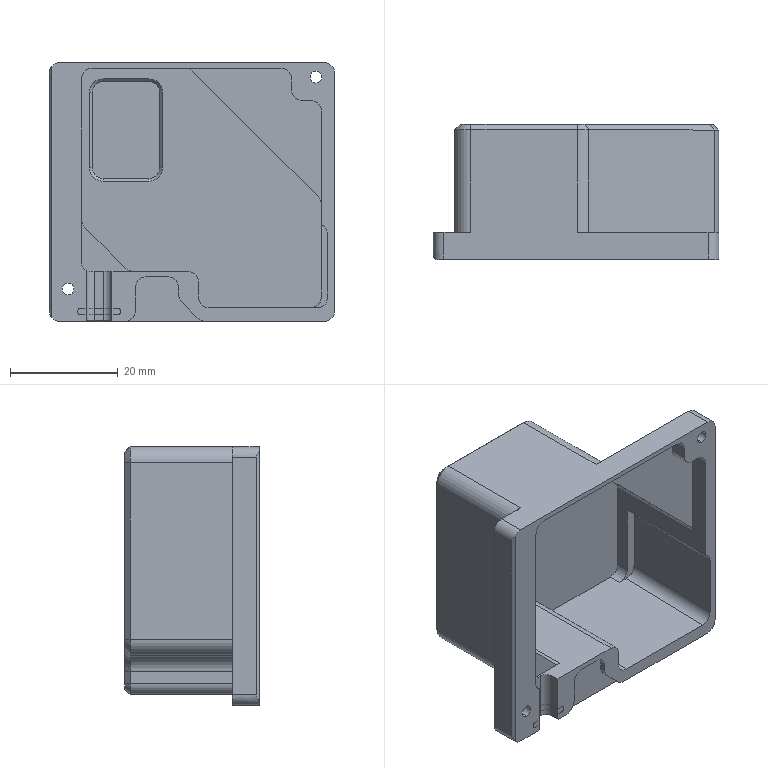NC program | NX | posted with a generic post | part box 53 x 25 x 48 mm
Whole program:
N10 G17 G21 G94 G90
(ZLEVEL_PROFILE_STEEP , TOOL : D4-12-D4-50-3T-ROUGH)
N12 T09 M6
N14 G54
N16 G17 G0 G90 X17.5 Y-7.5 B0. C0. S4000 M3
N18 G43 Z31.374 H9
N20 Z1.115 B-180. C178.5
N22 G94 G1 Z0.115 F1500.
N24 X18.3
N26 G3 X19.5 Y-6.3 R1.2
N28 G1 Y-4.39
N30 Y-3.37 Z0.068
N32 Y-3.297 Z0.065
N34 Y-6.3
N36 Z0.015
N38 Y-3.3
N40 X19.495
N42 X7.834
N44 Z-0.035
N46 X19.495
N48 X19.5
N50 Y-6.3
N52 Z-0.085
N54 Y-3.3
N56 X19.495
N58 X7.835
N60 Z-0.135
N62 X19.495
N64 X19.5
N66 Y-6.3
N68 Z-0.185
N70 Y-3.3
N72 X19.495
N74 X7.836
N76 Z-0.235
N78 X19.495
N80 X19.5
N82 Y-6.3
N84 Z-0.285
N86 Y-3.3
N88 X19.495
N90 X7.837
N92 Z-0.335
N94 X19.495
N96 X19.5
N98 Y-6.3
N100 Z-0.385
N102 Y-3.3
N104 X19.495
N106 X7.838
N108 Z-0.435
N110 X19.495
N112 X19.5
N114 Y-6.3
N116 Z-0.485
N118 Y-3.3
N120 X19.495
N122 X7.839
N124 X7.84 Z-0.535
N126 X19.495
N128 X19.5
N130 Y-6.3
N132 Z-0.585
N134 Y-3.3
N136 X19.495
N138 X7.84
N140 X7.841 Z-0.634
N142 X19.495
N144 X19.5
N146 Y-6.3
N148 Z-0.684
N150 Y-3.3
N152 X19.495
N154 X7.841
N156 X7.842 Z-0.734
N158 X19.495
N160 X19.5
N162 Y-6.3
N164 Z-0.784
N166 Y-3.3
N168 X19.495
N170 X7.842
N172 X7.843 Z-0.834
N174 X19.495
N176 X19.5
N178 Y-6.3
N180 Z-0.884
N182 Y-3.3
N184 X19.495
N186 X7.843
N188 X7.844 Z-0.934
N190 X19.495
N192 X19.5
N194 Y-6.3
N196 Z-0.984
N198 Y-3.3
N200 X19.495
N202 X7.844
N204 X7.845 Z-1.034
N206 X19.495
N208 X19.5
N210 Y-6.3
N212 Z-1.084
N214 Y-3.3
N216 X19.495
N218 X7.845
N220 X7.846 Z-1.134
N222 X19.495
N224 X19.5
N226 Y-6.3
N228 Z-1.184
N230 Y-3.3
N232 X19.495
N234 X7.847
N236 Z-1.234
N238 X19.495
N240 X19.5
N242 Y-6.3
N244 Z-1.284
N246 Y-3.3
N248 X19.495
N250 X7.848
N252 Z-1.334
N254 X19.495
N256 X19.5
N258 Y-6.3
N260 Z-1.384
N262 Y-3.3
N264 X19.495
N266 X7.849
N268 Z-1.434
N270 X19.495
N272 X19.5
N274 Y-6.3
N276 Z-1.484
N278 Y-3.3
N280 X19.495
N282 X7.85
N284 Z-1.534
N286 X19.495
N288 X19.5
N290 Y-6.3
N292 Z-1.584
N294 Y-3.3
N296 X19.495
N298 X7.851
N300 Z-1.634
N302 X19.495
N304 X19.5
N306 Y-6.3
N308 Z-1.684
N310 Y-3.3
N312 X19.495
N314 X7.852
N316 X7.853 Z-1.734
N318 X19.495
N320 X19.5
N322 Y-6.3
N324 Z-1.784
N326 Y-3.3
N328 X19.495
N330 X7.853
N332 X7.854 Z-1.834
N334 X19.495
N336 X19.5
N338 Y-6.3
N340 Z-1.884
N342 Y-3.3
N344 X19.495
N346 X7.854
N348 X7.855 Z-1.934
N350 X19.495
N352 X19.5
N354 Y-6.3
N356 Z-1.983
N358 Y-3.3
N360 X19.495
N362 X7.855
N364 X7.856 Z-2.033
N366 X19.495
N368 X19.5
N370 Y-6.3
N372 Z-2.083
N374 Y-3.3
N376 X19.495
N378 X7.856
N380 X7.857 Z-2.133
N382 X19.495
N384 X19.5
N386 Y-6.3
N388 Z-2.183
N390 Y-3.3
N392 X19.495
N394 X7.857
N396 X7.858 Z-2.233
N398 X19.495
N400 X19.5 Y-3.301
N402 Y-6.3
N404 Z-2.283
N406 Y-3.301
N408 X19.495 Y-3.3
N410 X7.859
N412 Z-2.333
N414 X19.495
N416 X19.5 Y-3.301
N418 Y-6.3
N420 Z-2.383
N422 Y-3.301
N424 X19.495 Y-3.3
N426 X7.86
N428 Z-2.433
N430 X19.495
N432 X19.5 Y-3.301
N434 Y-6.3
N436 Z-2.483
N438 Y-3.301
N440 X19.495 Y-3.3
N442 X7.861
N444 Z-2.533
N446 X19.495
N448 X19.5 Y-3.301
N450 Y-6.3
N452 Z-2.583
N454 Y-3.301
N456 X19.495 Y-3.3
N458 X7.862
N460 Z-2.633
N462 X19.495
N464 X19.5 Y-3.301
N466 Y-6.3
N468 Z-2.683
N470 Y-3.301
N472 X19.495 Y-3.3
N474 X7.863
N476 Z-2.733
N478 X19.495
N480 X19.5 Y-3.301
N482 Y-6.3
N484 Z-2.783
N486 Y-3.301
N488 X19.495 Y-3.3
N490 X7.864
N492 Z-2.833
N494 X19.495
N496 X19.5 Y-3.301
N498 Y-6.3
N500 Z-2.883
N502 Y-3.301
N504 X19.495 Y-3.3
N506 X7.865
N508 Z-2.933
N510 X19.495
N512 X19.5 Y-3.301
N514 Y-6.3
N516 Z-2.983
N518 Y-3.301
N520 X19.495 Y-3.3
N522 X7.866
N524 Z-3.033
N526 X19.495
N528 X19.5 Y-3.301
N530 Y-6.3
N532 Z-3.083
N534 Y-3.301
N536 X19.495 Y-3.3
N538 X7.867
N540 Z-3.133
N542 X19.495
N544 X19.5 Y-3.301
N546 Y-6.3
N548 Z-3.183
N550 Y-3.301
N552 X19.495 Y-3.3
N554 X7.868
N556 Z-3.233
N558 X19.495
N560 X19.5 Y-3.301
N562 Y-6.3
N564 Z-3.282
N566 Y-3.301
N568 X19.495 Y-3.3
N570 X7.869
N572 Z-3.332
N574 X19.495
N576 X19.5 Y-3.301
N578 Y-6.3
N580 Z-3.382
N582 Y-3.301
N584 X19.495 Y-3.3
N586 X7.87
N588 Z-3.432
N590 X19.495
N592 X19.5 Y-3.301
N594 Y-6.3
N596 Z-3.482
N598 Y-3.301
N600 X19.495 Y-3.3
N602 X7.87
N604 X7.871 Z-3.532
N606 X19.495
N608 X19.5 Y-3.301
N610 Y-6.3
N612 Z-3.582
N614 Y-3.301
N616 X19.495 Y-3.3
N618 X7.871
N620 X7.872 Z-3.632
N622 X19.495
N624 X19.5 Y-3.301
N626 Y-6.3
N628 Z-3.682
N630 Y-3.301
N632 X19.495 Y-3.3
N634 X7.872
N636 X7.873 Z-3.732
N638 X19.495
N640 X19.5 Y-3.301
N642 Y-6.3
N644 Z-3.782
N646 Y-3.301
N648 X19.495 Y-3.3
N650 X7.873
N652 X7.874 Z-3.832
N654 X19.495
N656 X19.5 Y-3.301
N658 Y-6.3
N660 Z-3.882
N662 Y-3.301
N664 X19.495 Y-3.3
N666 X7.874
N668 X7.875 Z-3.932
N670 X19.495
N672 X19.5 Y-3.301
N674 Y-6.3
N676 Z-3.982
N678 Y-3.301
N680 X19.495 Y-3.3
N682 X7.875
N684 X7.876 Z-4.032
N686 X19.495
N688 X19.5 Y-3.301
N690 Y-6.3
N692 Z-4.082
N694 Y-3.301
N696 X19.495 Y-3.3
N698 X7.876
N700 X7.877 Z-4.132
N702 X19.495
N704 X19.5 Y-3.301
N706 Y-6.3
N708 Z-4.182
N710 Y-3.301
N712 X19.495 Y-3.3
N714 X7.877
N716 X7.878 Z-4.232
N718 X19.495
N720 X19.5 Y-3.301
N722 Y-6.3
N724 Z-4.282
N726 Y-3.301
N728 X19.495 Y-3.3
N730 X7.878
N732 X7.879 Z-4.332
N734 X19.495
N736 X19.5 Y-3.301
N738 Y-6.3
N740 Z-4.382
N742 Y-3.301
N744 X19.495 Y-3.3
N746 X7.879
N748 X7.88 Z-4.432
N750 X19.495
N752 X19.5 Y-3.301
N754 Y-6.3
N756 Z-4.482
N758 Y-3.301
N760 X19.495 Y-3.3
N762 X7.88
N764 X7.881 Z-4.532
N766 X19.495
N768 X19.5 Y-3.301
N770 Y-6.3
N772 Z-4.582
N774 Y-3.301
N776 X19.495 Y-3.3
N778 X7.881
N780 X7.882 Z-4.631
N782 X19.495
N784 X19.5 Y-3.301
N786 Y-6.3
N788 Z-4.681
N790 Y-3.301
N792 X19.495 Y-3.3
N794 X7.882
N796 X7.883 Z-4.731
N798 X19.495
N800 X19.5 Y-3.301
N802 Y-6.3
N804 Z-4.781
N806 Y-3.301
N808 X19.495 Y-3.3
N810 X7.883
N812 X7.884 Z-4.831
N814 X19.495
N816 X19.5 Y-3.301
N818 Y-6.3
N820 Z-4.881
N822 Y-3.301
N824 X19.495 Y-3.3
N826 X7.884
N828 X7.885 Z-4.931
N830 X19.495
N832 X19.5 Y-3.301
N834 Y-6.3
N836 Z-4.981
N838 Y-3.301
N840 X19.495 Y-3.3
N842 X7.885
N844 X7.886 Z-5.031
N846 X19.495
N848 X19.5 Y-3.301
N850 Y-6.3
N852 Z-5.081
N854 Y-3.301
N856 X19.495 Y-3.3
N858 X7.886
N860 Z-5.131
N862 X19.495
N864 X19.5 Y-3.301
N866 Y-6.3
N868 Z-5.181
N870 Y-3.301
N872 X19.495 Y-3.3
N874 X7.887
N876 Z-5.231
N878 X19.495
N880 X19.5 Y-3.301
N882 Y-6.3
N884 Z-5.281
N886 Y-3.301
N888 X19.495 Y-3.3
N890 X7.888
N892 Z-5.331
N894 X19.495
N896 X19.5 Y-3.301
N898 Y-6.3
N900 Z-5.381
N902 Y-3.301
N904 X19.495 Y-3.3
N906 X7.889
N908 Z-5.431
N910 X19.495
N912 X19.5 Y-3.301
N914 Y-6.3
N916 Z-5.481
N918 Y-3.301
N920 X19.495 Y-3.3
N922 X7.89
N924 Z-5.531
N926 X19.495
N928 X19.5 Y-3.301
N930 Y-6.3
N932 Z-5.581
N934 Y-3.301
N936 X19.495 Y-3.3
N938 X7.89
N940 X7.891 Z-5.631
N942 X19.495
N944 X19.5 Y-3.301
N946 Y-6.3
N948 Z-5.681
N950 Y-3.301
N952 X19.495 Y-3.3
N954 X7.891
N956 X7.892 Z-5.731
N958 X19.495
N960 X19.5 Y-3.301
N962 Y-6.3
N964 Z-5.781
N966 Y-3.301
N968 X19.495 Y-3.3
N970 X7.892
N972 X7.893 Z-5.831
N974 X19.495
N976 X19.5 Y-3.301
N978 Y-6.3
N980 Z-5.881
N982 Y-3.301
N984 X19.495 Y-3.3
N986 X7.893
N988 X7.894 Z-5.931
N990 X19.495
N992 X19.5 Y-3.301
N994 Y-6.3
N996 Z-5.98
N998 Y-3.301
N1000 X19.495 Y-3.3
N1002 X7.894
N1004 Z-6.03
N1006 X19.495
N1008 X19.5 Y-3.301
N1010 Y-6.3
N1012 Z-6.08
N1014 Y-3.301
N1016 X19.495 Y-3.3
N1018 X7.895
N1020 Z-6.13
N1022 X19.495
N1024 X19.5 Y-3.301
N1026 Y-6.3
N1028 Z-6.18
N1030 Y-3.301
N1032 X19.495 Y-3.3
N1034 X7.896
N1036 Z-6.23
N1038 X19.495
N1040 X19.5 Y-3.301
N1042 Y-6.3
N1044 Z-6.28
N1046 Y-3.301
N1048 X19.495 Y-3.3
N1050 X7.897
N1052 Z-6.33
N1054 X19.495
N1056 X19.5 Y-3.301
N1058 Y-6.3
N1060 Z-6.38
N1062 Y-3.301
N1064 X19.495 Y-3.3
N1066 X7.898
N1068 Z-6.43
N1070 X19.495
N1072 X19.5 Y-3.301
N1074 Y-6.3
N1076 Z-6.48
N1078 Y-3.301
N1080 X19.495 Y-3.3
N1082 X7.898
N1084 X7.899 Z-6.53
N1086 X19.495
N1088 X19.5 Y-3.301
N1090 Y-6.3
N1092 Z-6.58
N1094 Y-3.301
N1096 X19.495 Y-3.3
N1098 X7.899
N1100 X7.9 Z-6.63
N1102 X19.495
N1104 X19.5 Y-3.301
N1106 Y-6.3
N1108 Z-6.68
N1110 Y-3.301
N1112 X19.495 Y-3.3
N1114 X7.9
N1116 X7.901 Z-6.73
N1118 X19.495
N1120 X19.5 Y-3.301
N1122 Y-6.3
N1124 Z-6.78
N1126 Y-3.301
N1128 X19.495 Y-3.3
N1130 X7.901
N1132 X7.902 Z-6.83
N1134 X19.495
N1136 X19.5 Y-3.301
N1138 Y-6.3
N1140 Z-6.88
N1142 Y-3.301
N1144 X19.495 Y-3.3
N1146 X7.902
N1148 Z-6.93
N1150 X19.495
N1152 X19.5 Y-3.301
N1154 Y-6.3
N1156 Z-6.98
N1158 Y-3.301
N1160 X19.495 Y-3.3
N1162 X7.903
N1164 Z-7.03
N1166 X19.495
N1168 X19.5 Y-3.301
N1170 Y-6.3
N1172 Z-7.08
N1174 Y-3.301
N1176 X19.495 Y-3.3
N1178 X7.904
N1180 Z-7.13
N1182 X19.495
N1184 X19.5 Y-3.301
N1186 Y-6.3
N1188 Z-7.18
N1190 Y-3.301
N1192 X19.495 Y-3.3
N1194 X7.905
N1196 Z-7.23
N1198 X19.495
N1200 X19.5 Y-3.301
N1202 Y-6.3
N1204 Z-7.28
N1206 Y-3.301
N1208 X19.495 Y-3.3
N1210 X7.905
N1212 X7.906 Z-7.329
N1214 X19.495
N1216 X19.5 Y-3.301
N1218 Y-6.3
N1220 Z-7.379
N1222 Y-3.301
N1224 X19.495 Y-3.3
N1226 X7.906
N1228 X7.907 Z-7.429
N1230 X19.495
N1232 X19.5 Y-3.301
N1234 Y-6.3
N1236 Z-7.479
N1238 Y-3.301
N1240 X19.495 Y-3.3
N1242 X7.907
N1244 Z-7.529
N1246 X19.495
N1248 X19.5 Y-3.301
N1250 Y-6.3
N1252 Z-7.579
N1254 Y-3.301
N1256 X19.495 Y-3.3
N1258 X7.908
N1260 Z-7.629
N1262 X19.495
N1264 X19.5 Y-3.301
N1266 Y-6.3
N1268 Z-7.679
N1270 Y-3.301
N1272 X19.495 Y-3.3
N1274 X7.909
N1276 Z-7.729
N1278 X19.495
N1280 X19.5 Y-3.301
N1282 Y-6.3
N1284 Z-7.779
N1286 Y-3.301
N1288 X19.495 Y-3.3
N1290 X7.909
N1292 X7.91 Z-7.829
N1294 X19.495
N1296 X19.5 Y-3.301
N1298 Y-6.3
N1300 Z-7.879
N1302 Y-3.301
N1304 X19.495 Y-3.3
N1306 X7.91
N1308 X7.911 Z-7.929
N1310 X19.495
N1312 X19.5 Y-3.301
N1314 Y-6.3
N1316 Z-7.979
N1318 Y-3.301
N1320 X19.495 Y-3.3
N1322 X7.911
N1324 Z-8.029
N1326 X19.495
N1328 X19.5 Y-3.301
N1330 Y-6.3
N1332 Z-8.079
N1334 Y-3.301
N1336 X19.495 Y-3.3
N1338 X7.912
N1340 Z-8.129
N1342 X19.495
N1344 X19.5 Y-3.301
N1346 Y-6.3
N1348 Z-8.179
N1350 Y-3.301
N1352 X19.495 Y-3.3
N1354 X7.913
N1356 Z-8.229
N1358 X19.495
N1360 X19.5 Y-3.301
N1362 Y-6.3
N1364 Z-8.279
N1366 Y-3.301
N1368 X19.495 Y-3.3
N1370 X7.913
N1372 X7.914 Z-8.329
N1374 X19.495
N1376 X19.5 Y-3.301
N1378 Y-6.3
N1380 Z-8.379
N1382 Y-3.301
N1384 X19.495 Y-3.3
N1386 X7.914
N1388 X7.915 Z-8.429
N1390 X19.495
N1392 X19.5 Y-3.301
N1394 Y-6.3
N1396 Z-8.479
N1398 Y-3.301
N1400 X19.495 Y-3.3
N1402 X7.915
N1404 Z-8.529
N1406 X19.495
N1408 X19.5 Y-3.301
N1410 Y-6.3
N1412 Z-8.579
N1414 Y-3.301
N1416 X19.495 Y-3.3
N1418 X7.916
N1420 Z-8.629
N1422 X19.495
N1424 X19.5 Y-3.301
N1426 Y-6.3
N1428 Z-8.678
N1430 Y-3.301
N1432 X19.495 Y-3.3
N1434 X7.917
N1436 Z-8.728
N1438 X19.495
N1440 X19.5 Y-3.301
N1442 Y-6.3
N1444 Z-8.778
N1446 Y-3.301
N1448 X19.495 Y-3.3
N1450 X7.917
N1452 X7.918 Z-8.828
N1454 X19.495
N1456 X19.5 Y-3.301
N1458 Y-6.3
N1460 Z-8.878
N1462 Y-3.301
N1464 X19.495 Y-3.3
N1466 X7.918
N1468 Z-8.928
N1470 X19.495
N1472 X19.5 Y-3.301
N1474 Y-6.3
N1476 Z-8.978
N1478 Y-3.301
N1480 X19.495 Y-3.3
N1482 X7.919
N1484 Z-9.028
N1486 X19.495
N1488 X19.5 Y-3.301
N1490 Y-6.3
N1492 Z-9.078
N1494 Y-3.301
N1496 X19.495 Y-3.3
N1498 X7.92
N1500 Z-9.128
N1502 X19.495
N1504 X19.5 Y-3.301
N1506 Y-6.3
N1508 Z-9.178
N1510 Y-3.301
N1512 X19.495 Y-3.3
N1514 X7.92
N1516 X7.921 Z-9.228
N1518 X19.495
N1520 X19.5 Y-3.301
N1522 Y-6.3
N1524 Z-9.278
N1526 Y-3.301
N1528 X19.495 Y-3.3
N1530 X7.921
N1532 X7.922 Z-9.328
N1534 X19.495
N1536 X19.5 Y-3.301
N1538 Y-6.3
N1540 Z-9.378
N1542 Y-3.301
N1544 X19.495 Y-3.3
N1546 X7.922
N1548 Z-9.428
N1550 X19.495
N1552 X19.5 Y-3.301
N1554 Y-6.3
N1556 Z-9.478
N1558 Y-3.301
N1560 X19.495 Y-3.3
N1562 X7.923
N1564 Z-9.528
N1566 X19.495
N1568 X19.5 Y-3.301
N1570 Y-6.3
N1572 Z-9.578
N1574 Y-3.301
N1576 X19.495 Y-3.3
N1578 X7.924
N1580 Z-9.628
N1582 X19.495
N1584 X19.5 Y-3.301
N1586 Y-6.3
N1588 Z-9.678
N1590 Y-3.301
N1592 X19.495 Y-3.3
N1594 X7.924
N1596 X7.925 Z-9.728
N1598 X19.495
N1600 X19.5 Y-3.301
N1602 Y-6.3
N1604 Z-9.778
N1606 Y-3.301
N1608 X19.495 Y-3.3
N1610 X7.925
N1612 Z-9.828
N1614 X19.495
N1616 X19.5 Y-3.301
N1618 Y-6.3
N1620 Z-9.878
N1622 Y-3.301
N1624 X19.495 Y-3.3
N1626 X7.926
N1628 Z-9.928
N1630 X19.495
N1632 X19.5 Y-3.301
N1634 Y-6.3
N1636 Z-9.977
N1638 Y-3.301
N1640 X19.495 Y-3.3
N1642 X7.927
N1644 Z-10.027
N1646 X19.495
N1648 X19.5 Y-3.301
N1650 Y-6.3
N1652 Z-10.077
N1654 Y-3.301
N1656 X19.495 Y-3.3
N1658 X7.927
N1660 X7.928 Z-10.127
N1662 X19.495
N1664 X19.5 Y-3.301
N1666 Y-6.3
N1668 Z-10.177
N1670 Y-3.301
N1672 X19.495 Y-3.3
N1674 X7.928
N1676 Z-10.227
N1678 X19.495
N1680 X19.5 Y-3.301
N1682 Y-6.3
N1684 Z-10.277
N1686 Y-3.301
N1688 X19.495 Y-3.3
N1690 X7.929
N1692 Z-10.327
N1694 X19.495
N1696 X19.5 Y-3.301
N1698 Y-6.3
N1700 Z-10.377
N1702 Y-3.301
N1704 X19.495 Y-3.3
N1706 X7.929
N1708 X7.93 Z-10.427
N1710 X19.495
N1712 X19.5 Y-3.301
N1714 Y-6.3
N1716 Z-10.477
N1718 Y-3.301
N1720 X19.495 Y-3.3
N1722 X7.93
N1724 Z-10.527
N1726 X19.495
N1728 X19.5 Y-3.301
N1730 Y-6.3
N1732 Z-10.577
N1734 Y-3.301
N1736 X19.495 Y-3.3
N1738 X7.931
N1740 Z-10.627
N1742 X19.495
N1744 X19.5 Y-3.301
N1746 Y-6.3
N1748 Z-10.677
N1750 Y-3.301
N1752 X19.495 Y-3.3
N1754 X7.931
N1756 X7.932 Z-10.727
N1758 X19.495
N1760 X19.5 Y-3.301
N1762 Y-6.3
N1764 Z-10.777
N1766 Y-3.301
N1768 X19.495 Y-3.3
N1770 X7.932
N1772 X7.933 Z-10.827
N1774 X19.495
N1776 X19.5 Y-3.301
N1778 Y-6.3
N1780 Z-10.877
N1782 Y-3.301
N1784 X19.495 Y-3.3
N1786 X7.933
N1788 Z-10.927
N1790 X19.495
N1792 X19.5 Y-3.301
N1794 Y-6.3
N1796 Z-10.977
N1798 Y-3.301
N1800 X19.495 Y-3.3
N1802 X7.934
N1804 Z-11.027
N1806 X19.495
N1808 X19.5 Y-3.301
N1810 Y-6.3
N1812 Z-11.077
N1814 Y-3.301
N1816 X19.495 Y-3.3
N1818 X7.934
N1820 X7.935 Z-11.127
N1822 X19.495
N1824 X19.5 Y-3.301
N1826 Y-6.3
N1828 Z-11.177
N1830 Y-3.301
N1832 X19.495 Y-3.3
N1834 X7.935
N1836 Z-11.227
N1838 X19.495
N1840 X19.5 Y-3.301
N1842 Y-6.3
N1844 Z-11.277
N1846 Y-3.301
N1848 X19.495 Y-3.3
N1850 X7.936
N1852 Z-11.326
N1854 X19.495
N1856 X19.5 Y-3.301
N1858 Y-6.3
N1860 Z-11.376
N1862 Y-3.301
N1864 X19.495 Y-3.3
N1866 X7.936
N1868 X7.937 Z-11.426
N1870 X19.495
N1872 X19.5 Y-3.301
N1874 Y-6.3
N1876 Z-11.476
N1878 Y-3.301
N1880 X19.495 Y-3.3
N1882 X7.937
N1884 Z-11.526
N1886 X19.495
N1888 X19.5 Y-3.301
N1890 Y-6.3
N1892 Z-11.576
N1894 Y-3.301
N1896 X19.495 Y-3.3
N1898 X7.938
N1900 Z-11.626
N1902 X19.495
N1904 X19.5 Y-3.301
N1906 Y-6.3
N1908 Z-11.676
N1910 Y-3.301
N1912 X19.495 Y-3.3
N1914 X7.938
N1916 X7.939 Z-11.726
N1918 X19.495
N1920 X19.5 Y-3.301
N1922 Y-6.3
N1924 Z-11.776
N1926 Y-3.301
N1928 X19.495 Y-3.3
N1930 X7.939
N1932 Z-11.826
N1934 X19.495
N1936 X19.5 Y-3.301
N1938 Y-6.3
N1940 Z-11.876
N1942 Y-3.301
N1944 X19.495 Y-3.3
N1946 X7.94
N1948 Z-11.926
N1950 X19.495
N1952 X19.5 Y-3.301
N1954 Y-6.3
N1956 Z-11.976
N1958 Y-3.301
N1960 X19.495 Y-3.3
N1962 X7.94
N1964 X7.941 Z-12.026
N1966 X19.495
N1968 X19.5 Y-3.301
N1970 Y-6.3
N1972 Z-12.076
N1974 Y-3.301
N1976 X19.495 Y-3.3
N1978 X7.941
N1980 Z-12.126
N1982 X19.495
N1984 X19.5 Y-3.301
N1986 Y-6.3
N1988 Z-12.176
N1990 Y-3.301
N1992 X19.495 Y-3.3
N1994 X7.942
N1996 Z-12.226
N1998 X19.495
N2000 X19.5 Y-3.301
N2002 Y-6.3
N2004 Z-12.276
N2006 Y-3.301
N2008 X19.495 Y-3.3
N2010 X7.942
N2012 X7.943 Z-12.326
N2014 X19.495
N2016 X19.5 Y-3.301
N2018 Y-6.3
N2020 Z-12.376
N2022 Y-3.301
N2024 X19.495 Y-3.3
N2026 X7.943
N2028 Z-12.426
N2030 X19.495
N2032 X19.5 Y-3.301
N2034 Y-6.3
N2036 Z-12.476
N2038 Y-3.301
N2040 X19.495 Y-3.3
N2042 X7.943
N2044 X7.944 Z-12.526
N2046 X19.495
N2048 X19.5 Y-3.301
N2050 Y-6.3
N2052 Z-12.576
N2054 Y-3.301
N2056 X19.495 Y-3.3
N2058 X7.944
N2060 Z-12.626
N2062 X19.495
N2064 X19.5 Y-3.301
N2066 Y-6.3
N2068 Z-12.675
N2070 Y-3.301
N2072 X19.495 Y-3.3
N2074 X7.945
N2076 Z-12.725
N2078 X19.495
N2080 X19.5 Y-3.301
N2082 Y-6.3
N2084 Z-12.775
N2086 Y-3.301
N2088 X19.495 Y-3.3
N2090 X7.945
N2092 X7.946 Z-12.825
N2094 X19.495
N2096 X19.5 Y-3.301
N2098 Y-6.3
N2100 Z-12.875
N2102 Y-3.301
N2104 X19.495 Y-3.3
N2106 X7.946
N2108 Z-12.925
N2110 X19.495
N2112 X19.5 Y-3.301
N2114 Y-6.3
N2116 Z-12.975
N2118 Y-3.301
N2120 X19.495 Y-3.3
N2122 X7.946
N2124 X7.947 Z-13.025
N2126 X19.495
N2128 X19.5 Y-3.301
N2130 Y-6.3
N2132 Z-13.075
N2134 Y-3.301
N2136 X19.495 Y-3.3
N2138 X7.947
N2140 Z-13.125
N2142 X19.495
N2144 X19.5 Y-3.301
N2146 Y-6.3
N2148 Z-13.175
N2150 Y-3.301
N2152 X19.495 Y-3.3
N2154 X7.948
N2156 Z-13.225
N2158 X19.495
N2160 X19.5 Y-3.301
N2162 Y-6.3
N2164 Z-13.275
N2166 Y-3.301
N2168 X19.495 Y-3.3
N2170 X7.948
N2172 X7.949 Z-13.325
N2174 X19.495
N2176 X19.5 Y-3.301
N2178 Y-6.3
N2180 Z-13.375
N2182 Y-3.301
N2184 X19.495 Y-3.3
N2186 X7.949
N2188 Z-13.425
N2190 X19.495
N2192 X19.5 Y-3.301
N2194 Y-6.3
N2196 Z-13.475
N2198 Y-3.301
N2200 X19.495 Y-3.3
N2202 X7.95
N2204 Z-13.525
N2206 X19.495
N2208 X19.5 Y-3.301
N2210 Y-6.3
N2212 Z-13.575
N2214 Y-3.301
N2216 X19.495 Y-3.3
N2218 X7.95
N2220 Z-13.625
N2222 X19.495
N2224 X19.5 Y-3.301
N2226 Y-6.3
N2228 Z-13.675
N2230 Y-3.301
N2232 X19.495 Y-3.3
N2234 X7.951
N2236 Z-13.725
N2238 X19.495
N2240 X19.5 Y-3.301
N2242 Y-6.3
N2244 Z-13.775
N2246 Y-3.301
N2248 X19.495 Y-3.3
N2250 X7.951
N2252 X7.952 Z-13.825
N2254 X19.495
N2256 X19.5 Y-3.301
N2258 Y-6.3
N2260 Z-13.875
N2262 Y-3.301
N2264 X19.495 Y-3.3
N2266 X7.952
N2268 Z-13.925
N2270 X19.495
N2272 X19.5 Y-3.301
N2274 Y-6.3
N2276 Z-13.975
N2278 Y-3.301
N2280 X19.495 Y-3.3
N2282 X7.953
N2284 Z-14.024
N2286 X19.495
N2288 X19.5 Y-3.301
N2290 Y-6.3
N2292 Z-14.074
N2294 Y-3.301
N2296 X19.495 Y-3.3
N2298 X7.953
N2300 Z-14.124
N2302 X19.495
N2304 X19.5 Y-3.301
N2306 Y-6.3
N2308 Z-14.174
N2310 Y-3.301
N2312 X19.495 Y-3.3
N2314 X7.954
N2316 Z-14.224
N2318 X19.495
N2320 X19.5 Y-3.301
N2322 Y-6.3
N2324 Z-14.274
N2326 Y-3.301
N2328 X19.495 Y-3.3
N2330 X7.954
N2332 X7.955 Z-14.324
N2334 X19.495
N2336 X19.5 Y-3.301
N2338 Y-6.3
N2340 Z-14.374
N2342 Y-3.301
N2344 X19.495 Y-3.3
N2346 X7.961
N2348 X7.955
N2350 Z-14.424
N2352 X7.956
N2354 X19.495
N2356 X19.5 Y-3.301
N2358 Y-6.3
N2360 Z-14.474
N2362 Y-3.301
N2364 X19.495 Y-3.3
N2366 X7.961
N2368 X7.956
N2370 Z-14.524
N2372 X19.495
N2374 X19.5 Y-3.301
N2376 Y-6.3
N2378 Z-14.574
N2380 Y-3.301
N2382 X19.495 Y-3.3
N2384 X7.961
N2386 Z-14.624
N2388 X19.495
N2390 X19.5 Y-3.301
N2392 Y-6.3
N2394 Z-14.674
N2396 Y-3.301
N2398 X19.495 Y-3.3
N2400 X7.961
N2402 Z-14.724
N2404 X19.495
N2406 X19.5 Y-3.301
N2408 Y-6.3
N2410 Z-14.774
N2412 Y-3.301
N2414 X19.495 Y-3.3
N2416 X7.961
N2418 Z-14.824
N2420 X19.495
N2422 X19.5 Y-3.301
N2424 Y-6.3
N2426 Z-14.874
N2428 Y-3.301
N2430 X19.495 Y-3.3
N2432 X7.961
N2434 Z-14.924
N2436 X19.495
N2438 X19.5 Y-3.301
N2440 Y-6.3
N2442 Z-14.974
N2444 Y-3.301
N2446 X19.495 Y-3.3
N2448 X7.961
N2450 Z-15.024
N2452 X19.495
N2454 X19.5 Y-3.301
N2456 Y-6.3
N2458 Z-15.074
N2460 Y-3.301
N2462 X19.495 Y-3.3
N2464 X7.961
N2466 Z-15.124
N2468 X19.495
N2470 X19.5 Y-3.301
N2472 Y-6.3
N2474 Z-15.174
N2476 Y-3.301
N2478 X19.495 Y-3.3
N2480 X7.961
N2482 Z-15.224
N2484 X19.495
N2486 X19.5 Y-3.301
N2488 Y-6.3
N2490 Z-15.274
N2492 Y-3.301
N2494 X19.495 Y-3.3
N2496 X7.961
N2498 Z-15.324
N2500 X19.495
N2502 X19.5 Y-3.301
N2504 Y-6.3
N2506 Z-15.373
N2508 Y-3.301
N2510 X19.495 Y-3.3
N2512 X7.961
N2514 Z-15.423
N2516 X19.495
N2518 X19.5 Y-3.301
N2520 Y-6.3
N2522 Z-15.473
N2524 Y-3.301
N2526 X19.495 Y-3.3
N2528 X7.961
N2530 Z-15.523
N2532 X19.495
N2534 X19.5 Y-3.301
N2536 Y-6.3
N2538 Z-15.573
N2540 Y-3.301
N2542 X19.495 Y-3.3
N2544 X7.961
N2546 X7.962 Z-15.623
N2548 X19.495
N2550 X19.5 Y-3.301
N2552 Y-6.3
N2554 Z-15.673
N2556 Y-3.301
N2558 X19.495 Y-3.3
N2560 X7.962
N2562 Z-15.723
N2564 X19.495
N2566 X19.5 Y-3.301
N2568 Y-6.3
N2570 Z-15.773
N2572 Y-3.301
N2574 X19.495 Y-3.3
N2576 X7.962
N2578 X7.963 Z-15.823
N2580 X19.495
N2582 X19.5 Y-3.301
N2584 Y-6.3
N2586 Z-15.873
N2588 Y-3.301
N2590 X19.495 Y-3.3
N2592 X7.963
N2594 Z-15.923
N2596 X19.495
N2598 X19.5 Y-3.301
N2600 Y-6.3
N2602 Z-15.973
N2604 Y-3.301
N2606 X19.495 Y-3.3
N2608 X7.963
N2610 X7.964 Z-16.023
N2612 X19.495
N2614 X19.5 Y-3.301
N2616 Y-6.3
N2618 Z-16.073
N2620 Y-3.301
N2622 X19.495 Y-3.3
N2624 X7.964
N2626 Z-16.123
N2628 X19.495
N2630 X19.5 Y-3.301
N2632 Y-6.3
N2634 Z-16.173
N2636 Y-3.301
N2638 X19.495 Y-3.3
N2640 X7.964
N2642 X7.965 Z-16.223
N2644 X19.495
N2646 X19.5 Y-3.301
N2648 Y-6.3
N2650 Z-16.273
N2652 Y-3.301
N2654 X19.495 Y-3.3
N2656 X7.965
N2658 Z-16.323
N2660 X19.495
N2662 X19.5 Y-3.301
N2664 Y-6.3
N2666 Z-16.373
N2668 Y-3.301
N2670 X19.495 Y-3.3
N2672 X7.965
N2674 X7.966 Z-16.423
N2676 X19.495
N2678 X19.5 Y-3.301
N2680 Y-6.3
N2682 Z-16.473
N2684 Y-3.301
N2686 X19.495 Y-3.3
N2688 X7.966
N2690 Z-16.523
N2692 X19.495
N2694 X19.5 Y-3.301
N2696 Y-6.3
N2698 Z-16.573
N2700 Y-3.301
N2702 X19.495 Y-3.3
N2704 X7.966
N2706 X7.967 Z-16.623
N2708 X19.495
N2710 X19.5 Y-3.301
N2712 Y-6.3
N2714 Z-16.672
N2716 Y-3.301
N2718 X19.495 Y-3.3
N2720 X7.967
N2722 Z-16.722
N2724 X19.495
N2726 X19.5 Y-3.301
N2728 Y-6.3
N2730 Z-16.772
N2732 Y-3.301
N2734 X19.495 Y-3.3
N2736 X7.967
N2738 X7.968 Z-16.822
N2740 X19.495
N2742 X19.5 Y-3.301
N2744 Y-6.3
N2746 Z-16.872
N2748 Y-3.301
N2750 X19.495 Y-3.3
N2752 X7.968
N2754 Z-16.922
N2756 X19.495
N2758 X19.5 Y-3.301
N2760 Y-6.3
N2762 Z-16.972
N2764 Y-3.301
N2766 X19.495 Y-3.3
N2768 X7.968
N2770 X7.969 Z-17.022
N2772 X19.495
N2774 X19.5 Y-3.301
N2776 Y-6.3
N2778 Z-17.072
N2780 Y-3.301
N2782 X19.495 Y-3.3
N2784 X7.969
N2786 Z-17.122
N2788 X19.495
N2790 X19.5 Y-3.301
N2792 Y-6.3
N2794 Z-17.172
N2796 Y-3.301
N2798 X19.495 Y-3.3
N2800 X7.969
N2802 X7.97 Z-17.222
N2804 X19.495
N2806 X19.5 Y-3.301
N2808 Y-6.3
N2810 Z-17.272
N2812 Y-3.301
N2814 X19.495 Y-3.3
N2816 X7.97
N2818 Z-17.322
N2820 X19.495
N2822 X19.5 Y-3.301
N2824 Y-6.3
N2826 Z-17.372
N2828 Y-3.301
N2830 X19.495 Y-3.3
N2832 X7.97
N2834 Z-17.422
N2836 X19.495
N2838 X19.5 Y-3.301
N2840 Y-6.3
N2842 Z-17.472
N2844 Y-3.301
N2846 X19.495 Y-3.3
N2848 X7.971
N2850 Z-17.522
N2852 X19.495
N2854 X19.5 Y-3.301
N2856 Y-6.3
N2858 Z-17.572
N2860 Y-3.301
N2862 X19.495 Y-3.3
N2864 X7.971
N2866 Z-17.622
N2868 X19.495
N2870 X19.5 Y-3.301
N2872 Y-6.3
N2874 Z-17.672
N2876 Y-3.301
N2878 X19.495 Y-3.3
N2880 X7.971
N2882 X7.972 Z-17.722
N2884 X19.495
N2886 X19.5 Y-3.301
N2888 Y-6.3
N2890 Z-17.772
N2892 Y-3.301
N2894 X19.495 Y-3.3
N2896 X7.972
N2898 Z-17.822
N2900 X19.495
N2902 X19.5 Y-3.301
N2904 Y-6.3
N2906 Z-17.872
N2908 Y-3.301
N2910 X19.495 Y-3.3
N2912 X7.972
N2914 X7.973 Z-17.922
N2916 X19.495
N2918 X19.5 Y-3.301
N2920 Y-6.3
N2922 Z-17.972
N2924 Y-3.301
N2926 X19.495 Y-3.3
N2928 X7.973
N2930 Z-18.021
N2932 X19.495
N2934 X19.5 Y-3.301
N2936 Y-6.3
N2938 Z-18.071
N2940 Y-3.301
N2942 X19.495 Y-3.3
N2944 X7.973
N2946 Z-18.121
N2948 X19.495
N2950 X19.5 Y-3.301
N2952 Y-6.3
N2954 Z-18.171
N2956 Y-3.301
N2958 X19.495 Y-3.3
N2960 X7.974
N2962 Z-18.221
N2964 X19.495
N2966 X19.5 Y-3.301
N2968 Y-6.3
N2970 Z-18.271
N2972 Y-3.301
N2974 X19.495 Y-3.3
N2976 X7.974
N2978 Z-18.321
N2980 X19.495
N2982 X19.5 Y-3.301
N2984 Y-6.3
N2986 Z-18.371
N2988 Y-3.301
N2990 X19.495 Y-3.3
N2992 X7.974
N2994 Z-18.421
N2996 X19.495
N2998 X19.5 Y-3.301
N3000 Y-6.3
N3002 Z-18.471
N3004 Y-3.301
N3006 X19.495 Y-3.3
N3008 X7.975
N3010 Z-18.521
N3012 X19.495
N3014 X19.5 Y-3.301
N3016 Y-6.3
N3018 Z-18.571
N3020 Y-3.301
N3022 X19.495 Y-3.3
N3024 X7.975
N3026 Z-18.621
N3028 X19.495
N3030 X19.5 Y-3.301
N3032 Y-6.3
N3034 Z-18.671
N3036 Y-3.301
N3038 X19.495 Y-3.3
N3040 X7.975
N3042 X7.976 Z-18.721
N3044 X19.495
N3046 X19.5 Y-3.301
N3048 Y-6.3
N3050 Z-18.771
N3052 Y-3.301
N3054 X19.495 Y-3.3
N3056 X7.976
N3058 Z-18.821
N3060 X19.495
N3062 X19.5 Y-3.301
N3064 Y-6.3
N3066 Z-18.871
N3068 Y-3.301
N3070 X19.495 Y-3.3
N3072 X7.976
N3074 Z-18.921
N3076 X19.495
N3078 X19.5 Y-3.301
N3080 Y-6.3
N3082 Z-18.971
N3084 Y-3.301
N3086 X19.495 Y-3.3
N3088 X7.977
N3090 Z-19.021
N3092 X19.495
N3094 X19.5 Y-3.301
N3096 Y-6.3
N3098 Z-19.071
N3100 Y-3.301
N3102 X19.495 Y-3.3
N3104 X7.977
N3106 Z-19.121
N3108 X19.495
N3110 X19.5 Y-3.301
N3112 Y-6.3
N3114 Z-19.171
N3116 Y-3.301
N3118 X19.495 Y-3.3
N3120 X7.977
N3122 X7.978 Z-19.221
N3124 X19.495
N3126 X19.5 Y-3.301
N3128 Y-6.3
N3130 Z-19.271
N3132 Y-3.301
N3134 X19.495 Y-3.3
N3136 X7.978
N3138 Z-19.321
N3140 X19.495
N3142 X19.5 Y-3.301
N3144 Y-6.3
N3146 Z-19.37
N3148 Y-3.301
N3150 X19.495 Y-3.3
N3152 X7.978
N3154 Z-19.42
N3156 X19.495
N3158 X19.5 Y-3.301
N3160 Y-6.3
N3162 Z-19.47
N3164 Y-3.301
N3166 X19.495 Y-3.3
N3168 X7.979
N3170 Z-19.52
N3172 X19.495
N3174 X19.5 Y-3.301
N3176 Y-6.3
N3178 Z-19.57
N3180 Y-3.301
N3182 X19.495 Y-3.3
N3184 X7.979
N3186 Z-19.62
N3188 X19.495
N3190 X19.5 Y-3.301
N3192 Y-6.3
N3194 Z-19.67
N3196 Y-3.301
N3198 X19.495 Y-3.3
N3200 X7.98
N3202 Z-19.72
N3204 X19.495
N3206 X19.5 Y-3.301
N3208 Y-6.3
N3210 Z-19.77
N3212 Y-3.301
N3214 X19.495 Y-3.3
N3216 X7.98
N3218 Z-19.82
N3220 X19.495
N3222 X19.5 Y-3.301
N3224 Y-6.3
N3226 Z-19.87
N3228 Y-3.301
N3230 X19.495 Y-3.3
N3232 X7.981
N3234 X7.98 Z-19.92
N3236 X19.495
N3238 X19.5 Y-3.301
N3240 Y-6.3
N3242 Z-19.97
N3244 Y-3.301
N3246 X19.495 Y-3.3
N3248 X7.981
N3250 Z-20.02
N3252 X19.495
N3254 X19.5 Y-3.301
N3256 Y-6.3
N3258 Z-20.07
N3260 Y-3.301
N3262 X19.495 Y-3.3
N3264 X7.981
N3266 Z-20.12
N3268 X19.495
N3270 X19.5 Y-3.301
N3272 Y-6.3
N3274 Z-20.17
N3276 Y-3.301
N3278 X19.495 Y-3.3
N3280 X7.981
N3282 X7.982 Z-20.22
N3284 X19.495
N3286 X19.5 Y-3.301
N3288 Y-6.3
N3290 Z-20.27
N3292 Y-3.301
N3294 X19.495 Y-3.3
N3296 X7.982
N3298 Z-20.32
N3300 X19.495
N3302 X19.5 Y-3.301
N3304 Y-6.3
N3306 Z-20.37
N3308 Y-3.301
N3310 X19.495 Y-3.3
N3312 X7.982
N3314 Z-20.42
N3316 X19.495
N3318 X19.5 Y-3.301
N3320 Y-5.21
N3322 Y-3.414 Z-20.47
N3324 Y-3.301
N3326 X19.495 Y-3.3
N3328 X7.983
N3330 X19.495
N3332 X19.5 Y-3.301
N3334 Y-3.414
N3336 G2 X18.3 Y-4.614 R1.2
N3338 G1 X17.5 Y-5.3
N3340 Z-19.47
N3342 G0 Z31.374
N3344 M5
N3346 M2